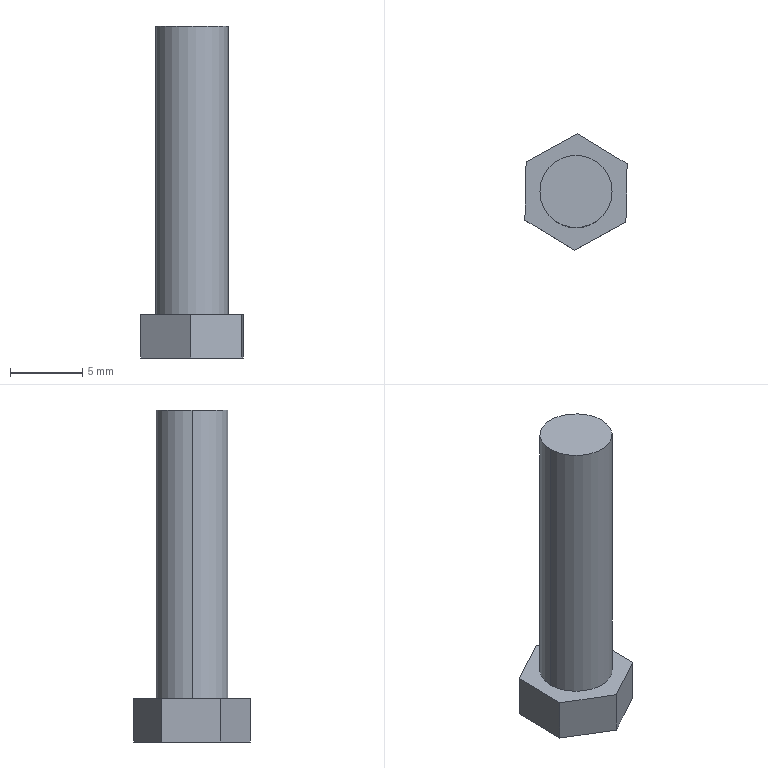Part | SolidWorks | features Extrusion 1, ICE 1 | 1 solid | 11 faces | box 7.081 x 8.081 x 23 mm | volume 520.005 mm3 | plane 9 | cylinder 2 | commonest cylinder face diameters 5 x2
STEP:
#1=CARTESIAN_POINT('',(2.5,0.,20.));
#2=VERTEX_POINT('',#1);
#3=CARTESIAN_POINT('',(-2.5,0.,20.));
#4=VERTEX_POINT('',#3);
#5=CARTESIAN_POINT('',(0.,0.,20.));
#6=DIRECTION('',(0.,0.,1.));
#7=DIRECTION('',(1.,0.,0.));
#8=AXIS2_PLACEMENT_3D('',#5,#6,#7);
#9=CIRCLE('',#8,2.5);
#10=EDGE_CURVE('',#2,#4,#9,.T.);
#11=ORIENTED_EDGE('',*,*,#10,.F.);
#12=CARTESIAN_POINT('',(2.5,0.,0.));
#13=VERTEX_POINT('',#12);
#14=CARTESIAN_POINT('',(2.5,0.,20.));
#15=DIRECTION('',(0.,0.,-1.));
#16=VECTOR('',#15,1000.);
#17=LINE('',#14,#16);
#18=EDGE_CURVE('',#2,#13,#17,.T.);
#19=ORIENTED_EDGE('',*,*,#18,.T.);
#20=CARTESIAN_POINT('',(-2.5,0.,0.));
#21=VERTEX_POINT('',#20);
#22=CARTESIAN_POINT('',(0.,0.,0.));
#23=DIRECTION('',(0.,0.,1.));
#24=DIRECTION('',(1.,0.,0.));
#25=AXIS2_PLACEMENT_3D('',#22,#23,#24);
#26=CIRCLE('',#25,2.5);
#27=EDGE_CURVE('',#13,#21,#26,.T.);
#28=ORIENTED_EDGE('',*,*,#27,.T.);
#29=CARTESIAN_POINT('',(-2.5,0.,20.));
#30=DIRECTION('',(0.,0.,-1.));
#31=VECTOR('',#30,1000.);
#32=LINE('',#29,#31);
#33=EDGE_CURVE('',#4,#21,#32,.T.);
#34=ORIENTED_EDGE('',*,*,#33,.F.);
#35=EDGE_LOOP('',(#11,#19,#28,#34));
#36=FACE_OUTER_BOUND('',#35,.T.);
#37=CARTESIAN_POINT('',(0.,0.,20.));
#38=DIRECTION('',(0.,0.,-1.));
#39=DIRECTION('',(-1.,0.,0.));
#40=AXIS2_PLACEMENT_3D('',#37,#38,#39);
#41=CYLINDRICAL_SURFACE('',#40,2.5);
#42=ADVANCED_FACE('',(#36),#41,.T.);
#43=ORIENTED_EDGE('',*,*,#18,.F.);
#44=CARTESIAN_POINT('',(0.,0.,20.));
#45=DIRECTION('',(0.,0.,1.));
#46=DIRECTION('',(1.,0.,0.));
#47=AXIS2_PLACEMENT_3D('',#44,#45,#46);
#48=CIRCLE('',#47,2.5);
#49=EDGE_CURVE('',#4,#2,#48,.T.);
#50=ORIENTED_EDGE('',*,*,#49,.F.);
#51=ORIENTED_EDGE('',*,*,#33,.T.);
#52=CARTESIAN_POINT('',(0.,0.,0.));
#53=DIRECTION('',(0.,0.,1.));
#54=DIRECTION('',(1.,0.,0.));
#55=AXIS2_PLACEMENT_3D('',#52,#53,#54);
#56=CIRCLE('',#55,2.5);
#57=EDGE_CURVE('',#21,#13,#56,.T.);
#58=ORIENTED_EDGE('',*,*,#57,.T.);
#59=EDGE_LOOP('',(#43,#50,#51,#58));
#60=FACE_OUTER_BOUND('',#59,.T.);
#61=CARTESIAN_POINT('',(0.,0.,20.));
#62=DIRECTION('',(0.,0.,-1.));
#63=DIRECTION('',(-1.,0.,0.));
#64=AXIS2_PLACEMENT_3D('',#61,#62,#63);
#65=CYLINDRICAL_SURFACE('',#64,2.5);
#66=ADVANCED_FACE('',(#60),#65,.T.);
#67=ORIENTED_EDGE('',*,*,#49,.T.);
#68=ORIENTED_EDGE('',*,*,#10,.T.);
#69=EDGE_LOOP('',(#67,#68));
#70=FACE_OUTER_BOUND('',#69,.T.);
#71=CARTESIAN_POINT('',(0.,0.,20.));
#72=DIRECTION('',(0.,0.,1.));
#73=DIRECTION('',(1.,0.,0.));
#74=AXIS2_PLACEMENT_3D('',#71,#72,#73);
#75=PLANE('',#74);
#76=ADVANCED_FACE('',(#70),#75,.T.);
#77=CARTESIAN_POINT('',(3.458,-2.092,0.));
#78=VERTEX_POINT('',#77);
#79=CARTESIAN_POINT('',(-0.08288,-4.041,0.));
#80=VERTEX_POINT('',#79);
#81=CARTESIAN_POINT('',(3.458,-2.092,0.));
#82=DIRECTION('',(-0.8761,-0.4821,0.));
#83=VECTOR('',#82,1000.);
#84=LINE('',#81,#83);
#85=EDGE_CURVE('',#78,#80,#84,.T.);
#86=ORIENTED_EDGE('',*,*,#85,.T.);
#87=CARTESIAN_POINT('',(-0.08288,-4.041,-3.));
#88=VERTEX_POINT('',#87);
#89=CARTESIAN_POINT('',(-0.08288,-4.041,-3.));
#90=DIRECTION('',(0.,0.,1.));
#91=VECTOR('',#90,1000.);
#92=LINE('',#89,#91);
#93=EDGE_CURVE('',#88,#80,#92,.T.);
#94=ORIENTED_EDGE('',*,*,#93,.F.);
#95=CARTESIAN_POINT('',(3.458,-2.092,-3.));
#96=VERTEX_POINT('',#95);
#97=CARTESIAN_POINT('',(3.458,-2.092,-3.));
#98=DIRECTION('',(-0.8761,-0.4821,0.));
#99=VECTOR('',#98,1000.);
#100=LINE('',#97,#99);
#101=EDGE_CURVE('',#96,#88,#100,.T.);
#102=ORIENTED_EDGE('',*,*,#101,.F.);
#103=CARTESIAN_POINT('',(3.458,-2.092,-3.));
#104=DIRECTION('',(0.,0.,1.));
#105=VECTOR('',#104,1000.);
#106=LINE('',#103,#105);
#107=EDGE_CURVE('',#96,#78,#106,.T.);
#108=ORIENTED_EDGE('',*,*,#107,.T.);
#109=EDGE_LOOP('',(#86,#94,#102,#108));
#110=FACE_OUTER_BOUND('',#109,.T.);
#111=CARTESIAN_POINT('',(3.458,-2.092,-3.));
#112=DIRECTION('',(-0.4821,0.8761,0.));
#113=DIRECTION('',(-0.8761,-0.4821,0.));
#114=AXIS2_PLACEMENT_3D('',#111,#112,#113);
#115=PLANE('',#114);
#116=ADVANCED_FACE('',(#110),#115,.F.);
#117=CARTESIAN_POINT('',(-3.541,-1.949,0.));
#118=VERTEX_POINT('',#117);
#119=CARTESIAN_POINT('',(-0.08288,-4.041,0.));
#120=DIRECTION('',(-0.8556,0.5177,0.));
#121=VECTOR('',#120,1000.);
#122=LINE('',#119,#121);
#123=EDGE_CURVE('',#80,#118,#122,.T.);
#124=ORIENTED_EDGE('',*,*,#123,.T.);
#125=CARTESIAN_POINT('',(-3.541,-1.949,-3.));
#126=VERTEX_POINT('',#125);
#127=CARTESIAN_POINT('',(-3.541,-1.949,-3.));
#128=DIRECTION('',(0.,0.,1.));
#129=VECTOR('',#128,1000.);
#130=LINE('',#127,#129);
#131=EDGE_CURVE('',#126,#118,#130,.T.);
#132=ORIENTED_EDGE('',*,*,#131,.F.);
#133=CARTESIAN_POINT('',(-0.08288,-4.041,-3.));
#134=DIRECTION('',(-0.8556,0.5177,0.));
#135=VECTOR('',#134,1000.);
#136=LINE('',#133,#135);
#137=EDGE_CURVE('',#88,#126,#136,.T.);
#138=ORIENTED_EDGE('',*,*,#137,.F.);
#139=ORIENTED_EDGE('',*,*,#93,.T.);
#140=EDGE_LOOP('',(#124,#132,#138,#139));
#141=FACE_OUTER_BOUND('',#140,.T.);
#142=CARTESIAN_POINT('',(-0.08288,-4.041,-3.));
#143=DIRECTION('',(0.5177,0.8556,0.));
#144=DIRECTION('',(-0.8556,0.5177,0.));
#145=AXIS2_PLACEMENT_3D('',#142,#143,#144);
#146=PLANE('',#145);
#147=ADVANCED_FACE('',(#141),#146,.F.);
#148=CARTESIAN_POINT('',(-3.458,2.092,0.));
#149=VERTEX_POINT('',#148);
#150=CARTESIAN_POINT('',(-3.541,-1.949,0.));
#151=DIRECTION('',(0.02051,0.9998,0.));
#152=VECTOR('',#151,1000.);
#153=LINE('',#150,#152);
#154=EDGE_CURVE('',#118,#149,#153,.T.);
#155=ORIENTED_EDGE('',*,*,#154,.T.);
#156=CARTESIAN_POINT('',(-3.458,2.092,-3.));
#157=VERTEX_POINT('',#156);
#158=CARTESIAN_POINT('',(-3.458,2.092,-3.));
#159=DIRECTION('',(0.,0.,1.));
#160=VECTOR('',#159,1000.);
#161=LINE('',#158,#160);
#162=EDGE_CURVE('',#157,#149,#161,.T.);
#163=ORIENTED_EDGE('',*,*,#162,.F.);
#164=CARTESIAN_POINT('',(-3.541,-1.949,-3.));
#165=DIRECTION('',(0.02051,0.9998,0.));
#166=VECTOR('',#165,1000.);
#167=LINE('',#164,#166);
#168=EDGE_CURVE('',#126,#157,#167,.T.);
#169=ORIENTED_EDGE('',*,*,#168,.F.);
#170=ORIENTED_EDGE('',*,*,#131,.T.);
#171=EDGE_LOOP('',(#155,#163,#169,#170));
#172=FACE_OUTER_BOUND('',#171,.T.);
#173=CARTESIAN_POINT('',(-3.541,-1.949,-3.));
#174=DIRECTION('',(0.9998,-0.02051,0.));
#175=DIRECTION('',(0.02051,0.9998,0.));
#176=AXIS2_PLACEMENT_3D('',#173,#174,#175);
#177=PLANE('',#176);
#178=ADVANCED_FACE('',(#172),#177,.F.);
#179=CARTESIAN_POINT('',(0.08288,4.041,0.));
#180=VERTEX_POINT('',#179);
#181=CARTESIAN_POINT('',(-3.458,2.092,0.));
#182=DIRECTION('',(0.8761,0.4821,0.));
#183=VECTOR('',#182,1000.);
#184=LINE('',#181,#183);
#185=EDGE_CURVE('',#149,#180,#184,.T.);
#186=ORIENTED_EDGE('',*,*,#185,.T.);
#187=CARTESIAN_POINT('',(0.08288,4.041,-3.));
#188=VERTEX_POINT('',#187);
#189=CARTESIAN_POINT('',(0.08288,4.041,-3.));
#190=DIRECTION('',(0.,0.,1.));
#191=VECTOR('',#190,1000.);
#192=LINE('',#189,#191);
#193=EDGE_CURVE('',#188,#180,#192,.T.);
#194=ORIENTED_EDGE('',*,*,#193,.F.);
#195=CARTESIAN_POINT('',(-3.458,2.092,-3.));
#196=DIRECTION('',(0.8761,0.4821,0.));
#197=VECTOR('',#196,1000.);
#198=LINE('',#195,#197);
#199=EDGE_CURVE('',#157,#188,#198,.T.);
#200=ORIENTED_EDGE('',*,*,#199,.F.);
#201=ORIENTED_EDGE('',*,*,#162,.T.);
#202=EDGE_LOOP('',(#186,#194,#200,#201));
#203=FACE_OUTER_BOUND('',#202,.T.);
#204=CARTESIAN_POINT('',(-3.458,2.092,-3.));
#205=DIRECTION('',(0.4821,-0.8761,0.));
#206=DIRECTION('',(0.8761,0.4821,0.));
#207=AXIS2_PLACEMENT_3D('',#204,#205,#206);
#208=PLANE('',#207);
#209=ADVANCED_FACE('',(#203),#208,.F.);
#210=CARTESIAN_POINT('',(3.541,1.949,0.));
#211=VERTEX_POINT('',#210);
#212=CARTESIAN_POINT('',(0.08288,4.041,0.));
#213=DIRECTION('',(0.8556,-0.5177,0.));
#214=VECTOR('',#213,1000.);
#215=LINE('',#212,#214);
#216=EDGE_CURVE('',#180,#211,#215,.T.);
#217=ORIENTED_EDGE('',*,*,#216,.T.);
#218=CARTESIAN_POINT('',(3.541,1.949,-3.));
#219=VERTEX_POINT('',#218);
#220=CARTESIAN_POINT('',(3.541,1.949,-3.));
#221=DIRECTION('',(0.,0.,1.));
#222=VECTOR('',#221,1000.);
#223=LINE('',#220,#222);
#224=EDGE_CURVE('',#219,#211,#223,.T.);
#225=ORIENTED_EDGE('',*,*,#224,.F.);
#226=CARTESIAN_POINT('',(0.08288,4.041,-3.));
#227=DIRECTION('',(0.8556,-0.5177,0.));
#228=VECTOR('',#227,1000.);
#229=LINE('',#226,#228);
#230=EDGE_CURVE('',#188,#219,#229,.T.);
#231=ORIENTED_EDGE('',*,*,#230,.F.);
#232=ORIENTED_EDGE('',*,*,#193,.T.);
#233=EDGE_LOOP('',(#217,#225,#231,#232));
#234=FACE_OUTER_BOUND('',#233,.T.);
#235=CARTESIAN_POINT('',(0.08288,4.041,-3.));
#236=DIRECTION('',(-0.5177,-0.8556,0.));
#237=DIRECTION('',(0.8556,-0.5177,0.));
#238=AXIS2_PLACEMENT_3D('',#235,#236,#237);
#239=PLANE('',#238);
#240=ADVANCED_FACE('',(#234),#239,.F.);
#241=CARTESIAN_POINT('',(3.541,1.949,0.));
#242=DIRECTION('',(-0.02051,-0.9998,0.));
#243=VECTOR('',#242,1000.);
#244=LINE('',#241,#243);
#245=EDGE_CURVE('',#211,#78,#244,.T.);
#246=ORIENTED_EDGE('',*,*,#245,.T.);
#247=ORIENTED_EDGE('',*,*,#107,.F.);
#248=CARTESIAN_POINT('',(3.541,1.949,-3.));
#249=DIRECTION('',(-0.02051,-0.9998,0.));
#250=VECTOR('',#249,1000.);
#251=LINE('',#248,#250);
#252=EDGE_CURVE('',#219,#96,#251,.T.);
#253=ORIENTED_EDGE('',*,*,#252,.F.);
#254=ORIENTED_EDGE('',*,*,#224,.T.);
#255=EDGE_LOOP('',(#246,#247,#253,#254));
#256=FACE_OUTER_BOUND('',#255,.T.);
#257=CARTESIAN_POINT('',(3.541,1.949,-3.));
#258=DIRECTION('',(-0.9998,0.02051,0.));
#259=DIRECTION('',(-0.02051,-0.9998,0.));
#260=AXIS2_PLACEMENT_3D('',#257,#258,#259);
#261=PLANE('',#260);
#262=ADVANCED_FACE('',(#256),#261,.F.);
#263=ORIENTED_EDGE('',*,*,#101,.T.);
#264=ORIENTED_EDGE('',*,*,#137,.T.);
#265=ORIENTED_EDGE('',*,*,#168,.T.);
#266=ORIENTED_EDGE('',*,*,#199,.T.);
#267=ORIENTED_EDGE('',*,*,#230,.T.);
#268=ORIENTED_EDGE('',*,*,#252,.T.);
#269=EDGE_LOOP('',(#263,#264,#265,#266,#267,#268));
#270=FACE_OUTER_BOUND('',#269,.T.);
#271=CARTESIAN_POINT('',(0.,0.,-3.));
#272=DIRECTION('',(0.,0.,-1.));
#273=DIRECTION('',(-1.,0.,0.));
#274=AXIS2_PLACEMENT_3D('',#271,#272,#273);
#275=PLANE('',#274);
#276=ADVANCED_FACE('',(#270),#275,.T.);
#277=ORIENTED_EDGE('',*,*,#57,.F.);
#278=ORIENTED_EDGE('',*,*,#27,.F.);
#279=EDGE_LOOP('',(#277,#278));
#280=FACE_BOUND('',#279,.T.);
#281=ORIENTED_EDGE('',*,*,#85,.F.);
#282=ORIENTED_EDGE('',*,*,#245,.F.);
#283=ORIENTED_EDGE('',*,*,#216,.F.);
#284=ORIENTED_EDGE('',*,*,#185,.F.);
#285=ORIENTED_EDGE('',*,*,#154,.F.);
#286=ORIENTED_EDGE('',*,*,#123,.F.);
#287=EDGE_LOOP('',(#281,#282,#283,#284,#285,#286));
#288=FACE_OUTER_BOUND('',#287,.T.);
#289=CARTESIAN_POINT('',(0.,0.,0.));
#290=DIRECTION('',(0.,0.,-1.));
#291=DIRECTION('',(-1.,0.,0.));
#292=AXIS2_PLACEMENT_3D('',#289,#290,#291);
#293=PLANE('',#292);
#294=ADVANCED_FACE('',(#280,#288),#293,.F.);
#295=CLOSED_SHELL('',(#42,#66,#76,#116,#147,#178,#209,#240,#262,#276,#294));
#296=MANIFOLD_SOLID_BREP('',#295);
#297=CARTESIAN_POINT('',(0.,0.,0.));
#298=DIRECTION('',(0.,0.,1.));
#299=DIRECTION('',(1.,0.,0.));
#300=AXIS2_PLACEMENT_3D('',#297,#298,#299);
#301=(LENGTH_UNIT()NAMED_UNIT(*)SI_UNIT(.MILLI.,.METRE.));
#302=UNCERTAINTY_MEASURE_WITH_UNIT(LENGTH_MEASURE(0.00001),#301,'','');
#303=(NAMED_UNIT(*)PLANE_ANGLE_UNIT()SI_UNIT($,.RADIAN.));
#304=(NAMED_UNIT(*)SI_UNIT($,.STERADIAN.)SOLID_ANGLE_UNIT());
#305=(GEOMETRIC_REPRESENTATION_CONTEXT(3)GLOBAL_UNCERTAINTY_ASSIGNED_CONTEXT((#302))GLOBAL_UNIT_ASSIGNED_CONTEXT((#301,#303,#304))REPRESENTATION_CONTEXT('',''));
#306=ADVANCED_BREP_SHAPE_REPRESENTATION('',(#296,#300),#305);